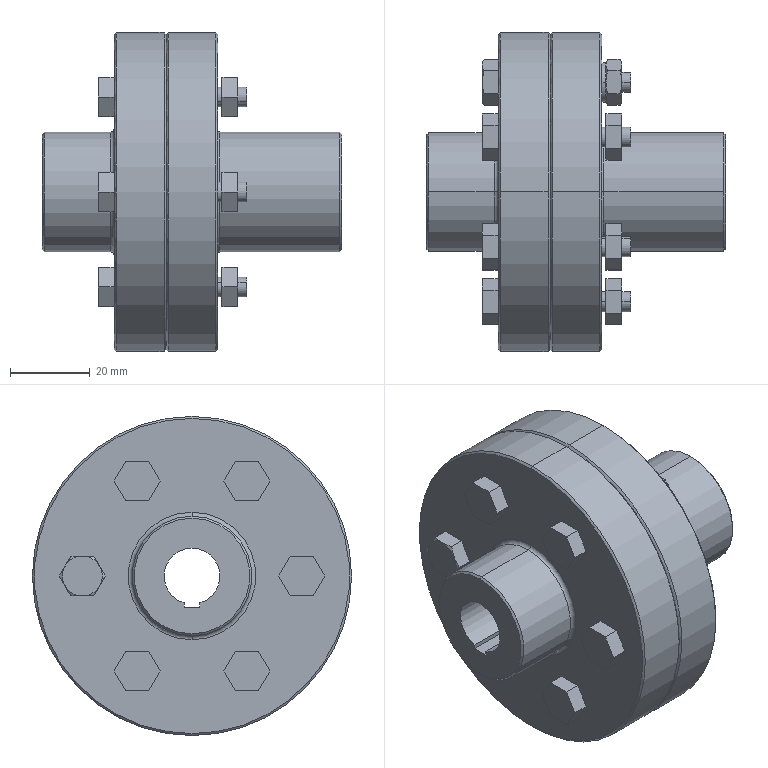Part | SolidWorks | features ICE 16, Chamfer 6, Revolution 3, CirPattern 2, Fillet 2, RefAxis 1 | 1 solid | 224 faces | box 75 x 80 x 80 mm | volume 155086 mm3 | plane 114 | cone 54 | cylinder 52 | torus 4 | commonest cylinder face diameters 5 x36 30 x6 80 x4 10 x2 14 x2 16 x2